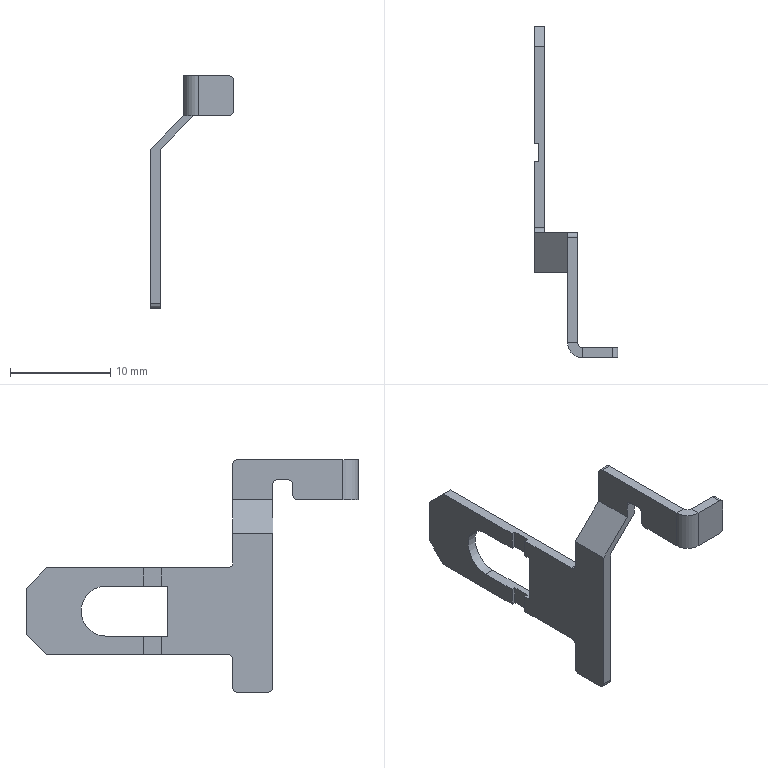Part | SolidWorks | features ICE 5, Chamfer 1, Fillet 1, FlatPattern 1, SMBaseFlange 1, SheetMetal 1 | 1 solid | 49 faces | box 8.33 x 33.1 x 23.2 mm | volume 267.226 mm3 | plane 36 | cylinder 13 | commonest cylinder face diameters 1 x11 3 x1 5 x1
STEP:
#1=CARTESIAN_POINT('',(-8.33,21.4,-8.6));
#2=VERTEX_POINT('',#1);
#3=CARTESIAN_POINT('',(-8.33,21.4,-6.8));
#4=VERTEX_POINT('',#3);
#5=CARTESIAN_POINT('',(-8.33,21.4,-19.2));
#6=DIRECTION('',(0.,0.,1.));
#7=VECTOR('',#6,1000.);
#8=LINE('',#5,#7);
#9=EDGE_CURVE('',#2,#4,#8,.T.);
#10=ORIENTED_EDGE('',*,*,#9,.F.);
#11=CARTESIAN_POINT('',(-7.93,21.4,-8.6));
#12=VERTEX_POINT('',#11);
#13=CARTESIAN_POINT('',(-8.33,21.4,-8.6));
#14=DIRECTION('',(1.,0.,0.));
#15=VECTOR('',#14,1000.);
#16=LINE('',#13,#15);
#17=EDGE_CURVE('',#2,#12,#16,.T.);
#18=ORIENTED_EDGE('',*,*,#17,.T.);
#19=CARTESIAN_POINT('',(-7.93,21.4,-6.8));
#20=VERTEX_POINT('',#19);
#21=CARTESIAN_POINT('',(-7.93,21.4,-19.2));
#22=DIRECTION('',(0.,0.,1.));
#23=VECTOR('',#22,1000.);
#24=LINE('',#21,#23);
#25=EDGE_CURVE('',#12,#20,#24,.T.);
#26=ORIENTED_EDGE('',*,*,#25,.T.);
#27=CARTESIAN_POINT('',(-8.33,21.4,-6.8));
#28=DIRECTION('',(-1.,0.,0.));
#29=VECTOR('',#28,1000.);
#30=LINE('',#27,#29);
#31=EDGE_CURVE('',#20,#4,#30,.T.);
#32=ORIENTED_EDGE('',*,*,#31,.T.);
#33=EDGE_LOOP('',(#10,#18,#26,#32));
#34=FACE_OUTER_BOUND('',#33,.T.);
#35=CARTESIAN_POINT('',(-8.33,21.4,-19.2));
#36=DIRECTION('',(0.,1.,0.));
#37=DIRECTION('',(-1.,0.,0.));
#38=AXIS2_PLACEMENT_3D('',#35,#36,#37);
#39=PLANE('',#38);
#40=ADVANCED_FACE('',(#34),#39,.F.);
#41=ORIENTED_EDGE('',*,*,#25,.F.);
#42=CARTESIAN_POINT('',(-7.93,19.6,-8.6));
#43=VERTEX_POINT('',#42);
#44=CARTESIAN_POINT('',(-7.93,21.4,-8.6));
#45=DIRECTION('',(0.,-1.,0.));
#46=VECTOR('',#45,1000.);
#47=LINE('',#44,#46);
#48=EDGE_CURVE('',#12,#43,#47,.T.);
#49=ORIENTED_EDGE('',*,*,#48,.T.);
#50=CARTESIAN_POINT('',(-7.93,19.6,-6.8));
#51=VERTEX_POINT('',#50);
#52=CARTESIAN_POINT('',(-7.93,19.6,-19.2));
#53=DIRECTION('',(0.,0.,1.));
#54=VECTOR('',#53,1000.);
#55=LINE('',#52,#54);
#56=EDGE_CURVE('',#43,#51,#55,.T.);
#57=ORIENTED_EDGE('',*,*,#56,.T.);
#58=CARTESIAN_POINT('',(-7.93,21.4,-6.8));
#59=DIRECTION('',(0.,1.,0.));
#60=VECTOR('',#59,1000.);
#61=LINE('',#58,#60);
#62=EDGE_CURVE('',#51,#20,#61,.T.);
#63=ORIENTED_EDGE('',*,*,#62,.T.);
#64=EDGE_LOOP('',(#41,#49,#57,#63));
#65=FACE_OUTER_BOUND('',#64,.T.);
#66=CARTESIAN_POINT('',(-7.93,21.4,-19.2));
#67=DIRECTION('',(1.,0.,0.));
#68=DIRECTION('',(0.,0.,-1.));
#69=AXIS2_PLACEMENT_3D('',#66,#67,#68);
#70=PLANE('',#69);
#71=ADVANCED_FACE('',(#65),#70,.F.);
#72=ORIENTED_EDGE('',*,*,#56,.F.);
#73=CARTESIAN_POINT('',(-8.33,19.6,-8.6));
#74=VERTEX_POINT('',#73);
#75=CARTESIAN_POINT('',(-8.33,19.6,-8.6));
#76=DIRECTION('',(-1.,0.,0.));
#77=VECTOR('',#76,1000.);
#78=LINE('',#75,#77);
#79=EDGE_CURVE('',#43,#74,#78,.T.);
#80=ORIENTED_EDGE('',*,*,#79,.T.);
#81=CARTESIAN_POINT('',(-8.33,19.6,-6.8));
#82=VERTEX_POINT('',#81);
#83=CARTESIAN_POINT('',(-8.33,19.6,-19.2));
#84=DIRECTION('',(0.,0.,1.));
#85=VECTOR('',#84,1000.);
#86=LINE('',#83,#85);
#87=EDGE_CURVE('',#74,#82,#86,.T.);
#88=ORIENTED_EDGE('',*,*,#87,.T.);
#89=CARTESIAN_POINT('',(-8.33,19.6,-6.8));
#90=DIRECTION('',(1.,0.,0.));
#91=VECTOR('',#90,1000.);
#92=LINE('',#89,#91);
#93=EDGE_CURVE('',#82,#51,#92,.T.);
#94=ORIENTED_EDGE('',*,*,#93,.T.);
#95=EDGE_LOOP('',(#72,#80,#88,#94));
#96=FACE_OUTER_BOUND('',#95,.T.);
#97=CARTESIAN_POINT('',(-8.33,19.6,-19.2));
#98=DIRECTION('',(0.,-1.,0.));
#99=DIRECTION('',(0.,0.,-1.));
#100=AXIS2_PLACEMENT_3D('',#97,#98,#99);
#101=PLANE('',#100);
#102=ADVANCED_FACE('',(#96),#101,.F.);
#103=CARTESIAN_POINT('',(-8.33,31.1,-6.8));
#104=VERTEX_POINT('',#103);
#105=CARTESIAN_POINT('',(-8.33,12.5,-6.8));
#106=DIRECTION('',(0.,1.,0.));
#107=VECTOR('',#106,1000.);
#108=LINE('',#105,#107);
#109=EDGE_CURVE('',#4,#104,#108,.T.);
#110=ORIENTED_EDGE('',*,*,#109,.T.);
#111=CARTESIAN_POINT('',(-8.33,33.1,-8.8));
#112=VERTEX_POINT('',#111);
#113=CARTESIAN_POINT('',(-8.33,26.,-1.7));
#114=DIRECTION('',(0.,0.7071,-0.7071));
#115=VECTOR('',#114,1000.);
#116=LINE('',#113,#115);
#117=EDGE_CURVE('',#104,#112,#116,.T.);
#118=ORIENTED_EDGE('',*,*,#117,.T.);
#119=CARTESIAN_POINT('',(-8.33,33.1,-13.4));
#120=VERTEX_POINT('',#119);
#121=CARTESIAN_POINT('',(-8.33,33.1,-15.4));
#122=DIRECTION('',(0.,0.,-1.));
#123=VECTOR('',#122,1000.);
#124=LINE('',#121,#123);
#125=EDGE_CURVE('',#112,#120,#124,.T.);
#126=ORIENTED_EDGE('',*,*,#125,.T.);
#127=CARTESIAN_POINT('',(-8.33,31.1,-15.4));
#128=VERTEX_POINT('',#127);
#129=CARTESIAN_POINT('',(-8.33,17.9,-28.6));
#130=DIRECTION('',(0.,-0.7071,-0.7071));
#131=VECTOR('',#130,1000.);
#132=LINE('',#129,#131);
#133=EDGE_CURVE('',#120,#128,#132,.T.);
#134=ORIENTED_EDGE('',*,*,#133,.T.);
#135=CARTESIAN_POINT('',(-8.33,21.4,-15.4));
#136=VERTEX_POINT('',#135);
#137=CARTESIAN_POINT('',(-8.33,12.5,-15.4));
#138=DIRECTION('',(0.,-1.,0.));
#139=VECTOR('',#138,1000.);
#140=LINE('',#137,#139);
#141=EDGE_CURVE('',#128,#136,#140,.T.);
#142=ORIENTED_EDGE('',*,*,#141,.T.);
#143=CARTESIAN_POINT('',(-8.33,21.4,-13.6));
#144=VERTEX_POINT('',#143);
#145=CARTESIAN_POINT('',(-8.33,21.4,-19.2));
#146=DIRECTION('',(0.,0.,1.));
#147=VECTOR('',#146,1000.);
#148=LINE('',#145,#147);
#149=EDGE_CURVE('',#136,#144,#148,.T.);
#150=ORIENTED_EDGE('',*,*,#149,.T.);
#151=CARTESIAN_POINT('',(-8.33,25.1,-13.6));
#152=VERTEX_POINT('',#151);
#153=CARTESIAN_POINT('',(-8.33,25.1,-13.6));
#154=DIRECTION('',(0.,-1.,0.));
#155=VECTOR('',#154,1000.);
#156=LINE('',#153,#155);
#157=EDGE_CURVE('',#152,#144,#156,.T.);
#158=ORIENTED_EDGE('',*,*,#157,.F.);
#159=CARTESIAN_POINT('',(-8.33,25.1,-8.6));
#160=VERTEX_POINT('',#159);
#161=CARTESIAN_POINT('',(-8.33,25.1,-11.1));
#162=DIRECTION('',(-1.,0.,0.));
#163=DIRECTION('',(0.,0.,1.));
#164=AXIS2_PLACEMENT_3D('',#161,#162,#163);
#165=CIRCLE('',#164,2.5);
#166=EDGE_CURVE('',#160,#152,#165,.T.);
#167=ORIENTED_EDGE('',*,*,#166,.F.);
#168=CARTESIAN_POINT('',(-8.33,25.1,-8.6));
#169=DIRECTION('',(0.,1.,0.));
#170=VECTOR('',#169,1000.);
#171=LINE('',#168,#170);
#172=EDGE_CURVE('',#2,#160,#171,.T.);
#173=ORIENTED_EDGE('',*,*,#172,.F.);
#174=ORIENTED_EDGE('',*,*,#9,.T.);
#175=EDGE_LOOP('',(#110,#118,#126,#134,#142,#150,#158,#167,#173,#174));
#176=FACE_OUTER_BOUND('',#175,.T.);
#177=CARTESIAN_POINT('',(-8.33,8.5,-19.2));
#178=DIRECTION('',(-1.,0.,0.));
#179=DIRECTION('',(0.,0.,1.));
#180=AXIS2_PLACEMENT_3D('',#177,#178,#179);
#181=PLANE('',#180);
#182=ADVANCED_FACE('',(#176),#181,.T.);
#183=CARTESIAN_POINT('',(-7.33,12.5,-3.33));
#184=VERTEX_POINT('',#183);
#185=CARTESIAN_POINT('',(-7.33,12.5,-6.3));
#186=VERTEX_POINT('',#185);
#187=CARTESIAN_POINT('',(-7.33,12.5,-3.33));
#188=DIRECTION('',(0.,0.,-1.));
#189=VECTOR('',#188,1000.);
#190=LINE('',#187,#189);
#191=EDGE_CURVE('',#184,#186,#190,.T.);
#192=ORIENTED_EDGE('',*,*,#191,.T.);
#193=CARTESIAN_POINT('',(-8.33,12.5,-6.3));
#194=VERTEX_POINT('',#193);
#195=CARTESIAN_POINT('',(-8.33,12.5,-6.3));
#196=DIRECTION('',(-1.,0.,0.));
#197=VECTOR('',#196,1000.);
#198=LINE('',#195,#197);
#199=EDGE_CURVE('',#186,#194,#198,.T.);
#200=ORIENTED_EDGE('',*,*,#199,.T.);
#201=CARTESIAN_POINT('',(-8.33,12.5,-3.33));
#202=VERTEX_POINT('',#201);
#203=CARTESIAN_POINT('',(-8.33,12.5,-19.2));
#204=DIRECTION('',(0.,0.,1.));
#205=VECTOR('',#204,1000.);
#206=LINE('',#203,#205);
#207=EDGE_CURVE('',#194,#202,#206,.T.);
#208=ORIENTED_EDGE('',*,*,#207,.T.);
#209=CARTESIAN_POINT('',(-5.,12.5,0.));
#210=VERTEX_POINT('',#209);
#211=CARTESIAN_POINT('',(-8.33,12.5,-3.33));
#212=DIRECTION('',(0.7071,0.,0.7071));
#213=VECTOR('',#212,1000.);
#214=LINE('',#211,#213);
#215=EDGE_CURVE('',#202,#210,#214,.T.);
#216=ORIENTED_EDGE('',*,*,#215,.T.);
#217=CARTESIAN_POINT('',(-5.,12.5,3.5));
#218=VERTEX_POINT('',#217);
#219=CARTESIAN_POINT('',(-5.,12.5,4.));
#220=DIRECTION('',(0.,0.,-1.));
#221=VECTOR('',#220,1000.);
#222=LINE('',#219,#221);
#223=EDGE_CURVE('',#218,#210,#222,.T.);
#224=ORIENTED_EDGE('',*,*,#223,.F.);
#225=CARTESIAN_POINT('',(-4.,12.5,3.5));
#226=VERTEX_POINT('',#225);
#227=CARTESIAN_POINT('',(-5.,12.5,3.5));
#228=DIRECTION('',(1.,0.,0.));
#229=VECTOR('',#228,1000.);
#230=LINE('',#227,#229);
#231=EDGE_CURVE('',#218,#226,#230,.T.);
#232=ORIENTED_EDGE('',*,*,#231,.T.);
#233=CARTESIAN_POINT('',(-4.,12.5,0.));
#234=VERTEX_POINT('',#233);
#235=CARTESIAN_POINT('',(-4.,12.5,4.));
#236=DIRECTION('',(0.,0.,-1.));
#237=VECTOR('',#236,1000.);
#238=LINE('',#235,#237);
#239=EDGE_CURVE('',#226,#234,#238,.T.);
#240=ORIENTED_EDGE('',*,*,#239,.T.);
#241=CARTESIAN_POINT('',(-4.,12.5,0.));
#242=DIRECTION('',(-0.7071,0.,-0.7071));
#243=VECTOR('',#242,1000.);
#244=LINE('',#241,#243);
#245=EDGE_CURVE('',#234,#184,#244,.T.);
#246=ORIENTED_EDGE('',*,*,#245,.T.);
#247=EDGE_LOOP('',(#192,#200,#208,#216,#224,#232,#240,#246));
#248=FACE_OUTER_BOUND('',#247,.T.);
#249=CARTESIAN_POINT('',(-5.,12.5,4.));
#250=DIRECTION('',(0.,1.,0.));
#251=DIRECTION('',(0.,0.,1.));
#252=AXIS2_PLACEMENT_3D('',#249,#250,#251);
#253=PLANE('',#252);
#254=ADVANCED_FACE('',(#248),#253,.T.);
#255=CARTESIAN_POINT('',(-5.,1.5,0.));
#256=VERTEX_POINT('',#255);
#257=CARTESIAN_POINT('',(-5.,6.,0.));
#258=VERTEX_POINT('',#257);
#259=CARTESIAN_POINT('',(-5.,0.,0.));
#260=DIRECTION('',(0.,1.,0.));
#261=VECTOR('',#260,1000.);
#262=LINE('',#259,#261);
#263=EDGE_CURVE('',#256,#258,#262,.T.);
#264=ORIENTED_EDGE('',*,*,#263,.T.);
#265=CARTESIAN_POINT('',(-4.,6.,0.));
#266=VERTEX_POINT('',#265);
#267=CARTESIAN_POINT('',(-3.5,6.,0.));
#268=DIRECTION('',(1.,0.,0.));
#269=VECTOR('',#268,1000.);
#270=LINE('',#267,#269);
#271=EDGE_CURVE('',#258,#266,#270,.T.);
#272=ORIENTED_EDGE('',*,*,#271,.T.);
#273=CARTESIAN_POINT('',(-4.,1.5,0.));
#274=VERTEX_POINT('',#273);
#275=CARTESIAN_POINT('',(-4.,0.,0.));
#276=DIRECTION('',(0.,1.,0.));
#277=VECTOR('',#276,1000.);
#278=LINE('',#275,#277);
#279=EDGE_CURVE('',#274,#266,#278,.T.);
#280=ORIENTED_EDGE('',*,*,#279,.F.);
#281=CARTESIAN_POINT('',(-4.,1.5,0.));
#282=DIRECTION('',(-1.,0.,0.));
#283=VECTOR('',#282,1000.);
#284=LINE('',#281,#283);
#285=EDGE_CURVE('',#274,#256,#284,.T.);
#286=ORIENTED_EDGE('',*,*,#285,.T.);
#287=EDGE_LOOP('',(#264,#272,#280,#286));
#288=FACE_OUTER_BOUND('',#287,.T.);
#289=CARTESIAN_POINT('',(-3.5,1.5,0.));
#290=DIRECTION('',(0.,0.,1.));
#291=DIRECTION('',(1.,0.,0.));
#292=AXIS2_PLACEMENT_3D('',#289,#290,#291);
#293=PLANE('',#292);
#294=ADVANCED_FACE('',(#288),#293,.F.);
#295=CARTESIAN_POINT('',(-5.,1.5,4.));
#296=VERTEX_POINT('',#295);
#297=CARTESIAN_POINT('',(-4.,1.5,4.));
#298=VERTEX_POINT('',#297);
#299=CARTESIAN_POINT('',(-5.,1.5,4.));
#300=DIRECTION('',(1.,0.,0.));
#301=VECTOR('',#300,1000.);
#302=LINE('',#299,#301);
#303=EDGE_CURVE('',#296,#298,#302,.T.);
#304=ORIENTED_EDGE('',*,*,#303,.F.);
#305=CARTESIAN_POINT('',(-3.5,0.,4.));
#306=VERTEX_POINT('',#305);
#307=CARTESIAN_POINT('',(-3.5,1.5,4.));
#308=DIRECTION('',(0.,0.,-1.));
#309=DIRECTION('',(1.,0.,0.));
#310=AXIS2_PLACEMENT_3D('',#307,#308,#309);
#311=CIRCLE('',#310,1.5);
#312=EDGE_CURVE('',#306,#296,#311,.T.);
#313=ORIENTED_EDGE('',*,*,#312,.F.);
#314=CARTESIAN_POINT('',(-3.5,1.,4.));
#315=VERTEX_POINT('',#314);
#316=CARTESIAN_POINT('',(-3.5,1.,4.));
#317=DIRECTION('',(0.,-1.,0.));
#318=VECTOR('',#317,1000.);
#319=LINE('',#316,#318);
#320=EDGE_CURVE('',#315,#306,#319,.T.);
#321=ORIENTED_EDGE('',*,*,#320,.F.);
#322=CARTESIAN_POINT('',(-3.5,1.5,4.));
#323=DIRECTION('',(0.,0.,-1.));
#324=DIRECTION('',(1.,0.,0.));
#325=AXIS2_PLACEMENT_3D('',#322,#323,#324);
#326=CIRCLE('',#325,0.5);
#327=EDGE_CURVE('',#315,#298,#326,.T.);
#328=ORIENTED_EDGE('',*,*,#327,.T.);
#329=EDGE_LOOP('',(#304,#313,#321,#328));
#330=FACE_OUTER_BOUND('',#329,.T.);
#331=CARTESIAN_POINT('',(-5.,1.5,4.));
#332=DIRECTION('',(0.,0.,1.));
#333=DIRECTION('',(1.,0.,0.));
#334=AXIS2_PLACEMENT_3D('',#331,#332,#333);
#335=PLANE('',#334);
#336=ADVANCED_FACE('',(#330),#335,.T.);
#337=CARTESIAN_POINT('',(-4.,12.,4.));
#338=VERTEX_POINT('',#337);
#339=CARTESIAN_POINT('',(-4.,0.,4.));
#340=DIRECTION('',(0.,1.,0.));
#341=VECTOR('',#340,1000.);
#342=LINE('',#339,#341);
#343=EDGE_CURVE('',#298,#338,#342,.T.);
#344=ORIENTED_EDGE('',*,*,#343,.T.);
#345=CARTESIAN_POINT('',(-5.,12.,4.));
#346=VERTEX_POINT('',#345);
#347=CARTESIAN_POINT('',(-3.5,12.,4.));
#348=DIRECTION('',(-1.,0.,0.));
#349=VECTOR('',#348,1000.);
#350=LINE('',#347,#349);
#351=EDGE_CURVE('',#338,#346,#350,.T.);
#352=ORIENTED_EDGE('',*,*,#351,.T.);
#353=CARTESIAN_POINT('',(-5.,0.,4.));
#354=DIRECTION('',(0.,1.,0.));
#355=VECTOR('',#354,1000.);
#356=LINE('',#353,#355);
#357=EDGE_CURVE('',#296,#346,#356,.T.);
#358=ORIENTED_EDGE('',*,*,#357,.F.);
#359=ORIENTED_EDGE('',*,*,#303,.T.);
#360=EDGE_LOOP('',(#344,#352,#358,#359));
#361=FACE_OUTER_BOUND('',#360,.T.);
#362=CARTESIAN_POINT('',(-3.5,1.,4.));
#363=DIRECTION('',(0.,0.,1.));
#364=DIRECTION('',(1.,0.,0.));
#365=AXIS2_PLACEMENT_3D('',#362,#363,#364);
#366=PLANE('',#365);
#367=ADVANCED_FACE('',(#361),#366,.T.);
#368=CARTESIAN_POINT('',(-3.5,0.,0.));
#369=VERTEX_POINT('',#368);
#370=CARTESIAN_POINT('',(-3.5,1.,0.));
#371=VERTEX_POINT('',#370);
#372=CARTESIAN_POINT('',(-3.5,0.,0.));
#373=DIRECTION('',(0.,1.,0.));
#374=VECTOR('',#373,1000.);
#375=LINE('',#372,#374);
#376=EDGE_CURVE('',#369,#371,#375,.T.);
#377=ORIENTED_EDGE('',*,*,#376,.F.);
#378=CARTESIAN_POINT('',(-3.5,1.5,0.));
#379=DIRECTION('',(0.,0.,-1.));
#380=DIRECTION('',(1.,0.,0.));
#381=AXIS2_PLACEMENT_3D('',#378,#379,#380);
#382=CIRCLE('',#381,1.5);
#383=EDGE_CURVE('',#369,#256,#382,.T.);
#384=ORIENTED_EDGE('',*,*,#383,.T.);
#385=ORIENTED_EDGE('',*,*,#285,.F.);
#386=CARTESIAN_POINT('',(-3.5,1.5,0.));
#387=DIRECTION('',(0.,0.,-1.));
#388=DIRECTION('',(1.,0.,0.));
#389=AXIS2_PLACEMENT_3D('',#386,#387,#388);
#390=CIRCLE('',#389,0.5);
#391=EDGE_CURVE('',#371,#274,#390,.T.);
#392=ORIENTED_EDGE('',*,*,#391,.F.);
#393=EDGE_LOOP('',(#377,#384,#385,#392));
#394=FACE_OUTER_BOUND('',#393,.T.);
#395=CARTESIAN_POINT('',(-3.5,0.,0.));
#396=DIRECTION('',(0.,0.,-1.));
#397=DIRECTION('',(-1.,0.,0.));
#398=AXIS2_PLACEMENT_3D('',#395,#396,#397);
#399=PLANE('',#398);
#400=ADVANCED_FACE('',(#394),#399,.T.);
#401=CARTESIAN_POINT('',(-0.5,1.,0.));
#402=VERTEX_POINT('',#401);
#403=CARTESIAN_POINT('',(0.,1.,0.));
#404=DIRECTION('',(-1.,0.,0.));
#405=VECTOR('',#404,1000.);
#406=LINE('',#403,#405);
#407=EDGE_CURVE('',#402,#371,#406,.T.);
#408=ORIENTED_EDGE('',*,*,#407,.F.);
#409=CARTESIAN_POINT('',(-0.5,0.,0.));
#410=VERTEX_POINT('',#409);
#411=CARTESIAN_POINT('',(-0.5,1.5,0.));
#412=DIRECTION('',(0.,-1.,0.));
#413=VECTOR('',#412,1000.);
#414=LINE('',#411,#413);
#415=EDGE_CURVE('',#402,#410,#414,.T.);
#416=ORIENTED_EDGE('',*,*,#415,.T.);
#417=CARTESIAN_POINT('',(0.,0.,0.));
#418=DIRECTION('',(-1.,0.,0.));
#419=VECTOR('',#418,1000.);
#420=LINE('',#417,#419);
#421=EDGE_CURVE('',#410,#369,#420,.T.);
#422=ORIENTED_EDGE('',*,*,#421,.T.);
#423=ORIENTED_EDGE('',*,*,#376,.T.);
#424=EDGE_LOOP('',(#408,#416,#422,#423));
#425=FACE_OUTER_BOUND('',#424,.T.);
#426=CARTESIAN_POINT('',(-4.,1.5,0.));
#427=DIRECTION('',(0.,0.,-1.));
#428=DIRECTION('',(-1.,0.,0.));
#429=AXIS2_PLACEMENT_3D('',#426,#427,#428);
#430=PLANE('',#429);
#431=ADVANCED_FACE('',(#425),#430,.T.);
#432=ORIENTED_EDGE('',*,*,#279,.T.);
#433=CARTESIAN_POINT('',(-4.,6.5,0.5));
#434=VERTEX_POINT('',#433);
#435=CARTESIAN_POINT('',(-4.,6.,0.5));
#436=DIRECTION('',(1.,0.,0.));
#437=DIRECTION('',(0.,0.,1.));
#438=AXIS2_PLACEMENT_3D('',#435,#436,#437);
#439=CIRCLE('',#438,0.5);
#440=EDGE_CURVE('',#266,#434,#439,.T.);
#441=ORIENTED_EDGE('',*,*,#440,.T.);
#442=CARTESIAN_POINT('',(-4.,6.5,1.5));
#443=VERTEX_POINT('',#442);
#444=CARTESIAN_POINT('',(-4.,6.5,4.));
#445=DIRECTION('',(0.,0.,1.));
#446=VECTOR('',#445,1000.);
#447=LINE('',#444,#446);
#448=EDGE_CURVE('',#434,#443,#447,.T.);
#449=ORIENTED_EDGE('',*,*,#448,.T.);
#450=CARTESIAN_POINT('',(-4.,7.,2.));
#451=VERTEX_POINT('',#450);
#452=CARTESIAN_POINT('',(-4.,7.,1.5));
#453=DIRECTION('',(-1.,0.,0.));
#454=DIRECTION('',(0.,0.,1.));
#455=AXIS2_PLACEMENT_3D('',#452,#453,#454);
#456=CIRCLE('',#455,0.5);
#457=EDGE_CURVE('',#443,#451,#456,.T.);
#458=ORIENTED_EDGE('',*,*,#457,.T.);
#459=CARTESIAN_POINT('',(-4.,8.,2.));
#460=VERTEX_POINT('',#459);
#461=CARTESIAN_POINT('',(-4.,0.,2.));
#462=DIRECTION('',(0.,1.,0.));
#463=VECTOR('',#462,1000.);
#464=LINE('',#461,#463);
#465=EDGE_CURVE('',#451,#460,#464,.T.);
#466=ORIENTED_EDGE('',*,*,#465,.T.);
#467=CARTESIAN_POINT('',(-4.,8.5,1.5));
#468=VERTEX_POINT('',#467);
#469=CARTESIAN_POINT('',(-4.,8.,1.5));
#470=DIRECTION('',(-1.,0.,0.));
#471=DIRECTION('',(0.,0.,1.));
#472=AXIS2_PLACEMENT_3D('',#469,#470,#471);
#473=CIRCLE('',#472,0.5);
#474=EDGE_CURVE('',#460,#468,#473,.T.);
#475=ORIENTED_EDGE('',*,*,#474,.T.);
#476=CARTESIAN_POINT('',(-4.,8.5,0.));
#477=VERTEX_POINT('',#476);
#478=CARTESIAN_POINT('',(-4.,8.5,4.));
#479=DIRECTION('',(0.,0.,-1.));
#480=VECTOR('',#479,1000.);
#481=LINE('',#478,#480);
#482=EDGE_CURVE('',#468,#477,#481,.T.);
#483=ORIENTED_EDGE('',*,*,#482,.T.);
#484=CARTESIAN_POINT('',(-4.,8.5,0.));
#485=DIRECTION('',(0.,1.,0.));
#486=VECTOR('',#485,1000.);
#487=LINE('',#484,#486);
#488=EDGE_CURVE('',#477,#234,#487,.T.);
#489=ORIENTED_EDGE('',*,*,#488,.T.);
#490=ORIENTED_EDGE('',*,*,#239,.F.);
#491=CARTESIAN_POINT('',(-4.,12.,3.5));
#492=DIRECTION('',(1.,0.,0.));
#493=DIRECTION('',(0.,0.,1.));
#494=AXIS2_PLACEMENT_3D('',#491,#492,#493);
#495=CIRCLE('',#494,0.5);
#496=EDGE_CURVE('',#226,#338,#495,.T.);
#497=ORIENTED_EDGE('',*,*,#496,.T.);
#498=ORIENTED_EDGE('',*,*,#343,.F.);
#499=CARTESIAN_POINT('',(-4.,1.5,4.));
#500=DIRECTION('',(0.,0.,-1.));
#501=VECTOR('',#500,1000.);
#502=LINE('',#499,#501);
#503=EDGE_CURVE('',#298,#274,#502,.T.);
#504=ORIENTED_EDGE('',*,*,#503,.T.);
#505=EDGE_LOOP('',(#432,#441,#449,#458,#466,#475,#483,#489,#490,#497,#498,#504));
#506=FACE_OUTER_BOUND('',#505,.T.);
#507=CARTESIAN_POINT('',(-4.,0.,4.));
#508=DIRECTION('',(-1.,0.,0.));
#509=DIRECTION('',(0.,0.,1.));
#510=AXIS2_PLACEMENT_3D('',#507,#508,#509);
#511=PLANE('',#510);
#512=ADVANCED_FACE('',(#506),#511,.F.);
#513=CARTESIAN_POINT('',(-8.33,12.5,-18.7));
#514=VERTEX_POINT('',#513);
#515=CARTESIAN_POINT('',(-8.33,12.5,-15.9));
#516=VERTEX_POINT('',#515);
#517=CARTESIAN_POINT('',(-8.33,12.5,-19.2));
#518=DIRECTION('',(0.,0.,1.));
#519=VECTOR('',#518,1000.);
#520=LINE('',#517,#519);
#521=EDGE_CURVE('',#514,#516,#520,.T.);
#522=ORIENTED_EDGE('',*,*,#521,.T.);
#523=CARTESIAN_POINT('',(-7.33,12.5,-15.9));
#524=VERTEX_POINT('',#523);
#525=CARTESIAN_POINT('',(-7.33,12.5,-15.9));
#526=DIRECTION('',(1.,0.,0.));
#527=VECTOR('',#526,1000.);
#528=LINE('',#525,#527);
#529=EDGE_CURVE('',#516,#524,#528,.T.);
#530=ORIENTED_EDGE('',*,*,#529,.T.);
#531=CARTESIAN_POINT('',(-7.33,12.5,-18.7));
#532=VERTEX_POINT('',#531);
#533=CARTESIAN_POINT('',(-7.33,12.5,-3.33));
#534=DIRECTION('',(0.,0.,-1.));
#535=VECTOR('',#534,1000.);
#536=LINE('',#533,#535);
#537=EDGE_CURVE('',#524,#532,#536,.T.);
#538=ORIENTED_EDGE('',*,*,#537,.T.);
#539=CARTESIAN_POINT('',(-5.,12.5,-18.7));
#540=DIRECTION('',(-1.,0.,0.));
#541=VECTOR('',#540,1000.);
#542=LINE('',#539,#541);
#543=EDGE_CURVE('',#532,#514,#542,.T.);
#544=ORIENTED_EDGE('',*,*,#543,.T.);
#545=EDGE_LOOP('',(#522,#530,#538,#544));
#546=FACE_OUTER_BOUND('',#545,.T.);
#547=CARTESIAN_POINT('',(-5.,12.5,4.));
#548=DIRECTION('',(0.,1.,0.));
#549=DIRECTION('',(0.,0.,1.));
#550=AXIS2_PLACEMENT_3D('',#547,#548,#549);
#551=PLANE('',#550);
#552=ADVANCED_FACE('',(#546),#551,.T.);
#553=CARTESIAN_POINT('',(-5.,6.5,0.5));
#554=VERTEX_POINT('',#553);
#555=CARTESIAN_POINT('',(-5.,6.5,1.5));
#556=VERTEX_POINT('',#555);
#557=CARTESIAN_POINT('',(-5.,6.5,0.));
#558=DIRECTION('',(0.,0.,1.));
#559=VECTOR('',#558,1000.);
#560=LINE('',#557,#559);
#561=EDGE_CURVE('',#554,#556,#560,.T.);
#562=ORIENTED_EDGE('',*,*,#561,.F.);
#563=CARTESIAN_POINT('',(-5.,6.,0.5));
#564=DIRECTION('',(-1.,0.,0.));
#565=DIRECTION('',(0.,0.,1.));
#566=AXIS2_PLACEMENT_3D('',#563,#564,#565);
#567=CIRCLE('',#566,0.5);
#568=EDGE_CURVE('',#554,#258,#567,.T.);
#569=ORIENTED_EDGE('',*,*,#568,.T.);
#570=ORIENTED_EDGE('',*,*,#263,.F.);
#571=CARTESIAN_POINT('',(-5.,1.5,4.));
#572=DIRECTION('',(0.,0.,-1.));
#573=VECTOR('',#572,1000.);
#574=LINE('',#571,#573);
#575=EDGE_CURVE('',#296,#256,#574,.T.);
#576=ORIENTED_EDGE('',*,*,#575,.F.);
#577=ORIENTED_EDGE('',*,*,#357,.T.);
#578=CARTESIAN_POINT('',(-5.,12.,3.5));
#579=DIRECTION('',(-1.,0.,0.));
#580=DIRECTION('',(0.,0.,1.));
#581=AXIS2_PLACEMENT_3D('',#578,#579,#580);
#582=CIRCLE('',#581,0.5);
#583=EDGE_CURVE('',#346,#218,#582,.T.);
#584=ORIENTED_EDGE('',*,*,#583,.T.);
#585=ORIENTED_EDGE('',*,*,#223,.T.);
#586=CARTESIAN_POINT('',(-5.,8.5,0.));
#587=VERTEX_POINT('',#586);
#588=CARTESIAN_POINT('',(-5.,8.5,0.));
#589=DIRECTION('',(0.,1.,0.));
#590=VECTOR('',#589,1000.);
#591=LINE('',#588,#590);
#592=EDGE_CURVE('',#587,#210,#591,.T.);
#593=ORIENTED_EDGE('',*,*,#592,.F.);
#594=CARTESIAN_POINT('',(-5.,8.5,1.5));
#595=VERTEX_POINT('',#594);
#596=CARTESIAN_POINT('',(-5.,8.5,0.));
#597=DIRECTION('',(0.,0.,-1.));
#598=VECTOR('',#597,1000.);
#599=LINE('',#596,#598);
#600=EDGE_CURVE('',#595,#587,#599,.T.);
#601=ORIENTED_EDGE('',*,*,#600,.F.);
#602=CARTESIAN_POINT('',(-5.,8.,2.));
#603=VERTEX_POINT('',#602);
#604=CARTESIAN_POINT('',(-5.,8.,1.5));
#605=DIRECTION('',(1.,0.,0.));
#606=DIRECTION('',(0.,0.,1.));
#607=AXIS2_PLACEMENT_3D('',#604,#605,#606);
#608=CIRCLE('',#607,0.5);
#609=EDGE_CURVE('',#595,#603,#608,.T.);
#610=ORIENTED_EDGE('',*,*,#609,.T.);
#611=CARTESIAN_POINT('',(-5.,7.,2.));
#612=VERTEX_POINT('',#611);
#613=CARTESIAN_POINT('',(-5.,8.5,2.));
#614=DIRECTION('',(0.,1.,0.));
#615=VECTOR('',#614,1000.);
#616=LINE('',#613,#615);
#617=EDGE_CURVE('',#612,#603,#616,.T.);
#618=ORIENTED_EDGE('',*,*,#617,.F.);
#619=CARTESIAN_POINT('',(-5.,7.,1.5));
#620=DIRECTION('',(1.,0.,0.));
#621=DIRECTION('',(0.,0.,1.));
#622=AXIS2_PLACEMENT_3D('',#619,#620,#621);
#623=CIRCLE('',#622,0.5);
#624=EDGE_CURVE('',#612,#556,#623,.T.);
#625=ORIENTED_EDGE('',*,*,#624,.T.);
#626=EDGE_LOOP('',(#562,#569,#570,#576,#577,#584,#585,#593,#601,#610,#618,#625));
#627=FACE_OUTER_BOUND('',#626,.T.);
#628=CARTESIAN_POINT('',(-5.,0.,4.));
#629=DIRECTION('',(-1.,0.,0.));
#630=DIRECTION('',(0.,0.,1.));
#631=AXIS2_PLACEMENT_3D('',#628,#629,#630);
#632=PLANE('',#631);
#633=ADVANCED_FACE('',(#627),#632,.T.);
#634=ORIENTED_EDGE('',*,*,#383,.F.);
#635=CARTESIAN_POINT('',(-3.5,0.,4.));
#636=DIRECTION('',(0.,0.,-1.));
#637=VECTOR('',#636,1000.);
#638=LINE('',#635,#637);
#639=EDGE_CURVE('',#306,#369,#638,.T.);
#640=ORIENTED_EDGE('',*,*,#639,.F.);
#641=ORIENTED_EDGE('',*,*,#312,.T.);
#642=ORIENTED_EDGE('',*,*,#575,.T.);
#643=EDGE_LOOP('',(#634,#640,#641,#642));
#644=FACE_OUTER_BOUND('',#643,.T.);
#645=CARTESIAN_POINT('',(-3.5,1.5,4.));
#646=DIRECTION('',(0.,0.,-1.));
#647=DIRECTION('',(-1.,0.,0.));
#648=AXIS2_PLACEMENT_3D('',#645,#646,#647);
#649=CYLINDRICAL_SURFACE('',#648,1.5);
#650=ADVANCED_FACE('',(#644),#649,.T.);
#651=CARTESIAN_POINT('',(0.,0.,3.5));
#652=VERTEX_POINT('',#651);
#653=CARTESIAN_POINT('',(0.,0.,0.5));
#654=VERTEX_POINT('',#653);
#655=CARTESIAN_POINT('',(0.,0.,4.));
#656=DIRECTION('',(0.,0.,-1.));
#657=VECTOR('',#656,1000.);
#658=LINE('',#655,#657);
#659=EDGE_CURVE('',#652,#654,#658,.T.);
#660=ORIENTED_EDGE('',*,*,#659,.F.);
#661=CARTESIAN_POINT('',(-0.5,0.,4.));
#662=VERTEX_POINT('',#661);
#663=CARTESIAN_POINT('',(-0.5,0.,3.5));
#664=DIRECTION('',(0.,-1.,0.));
#665=DIRECTION('',(0.,0.,-1.));
#666=AXIS2_PLACEMENT_3D('',#663,#664,#665);
#667=CIRCLE('',#666,0.5);
#668=EDGE_CURVE('',#652,#662,#667,.T.);
#669=ORIENTED_EDGE('',*,*,#668,.T.);
#670=CARTESIAN_POINT('',(0.,0.,4.));
#671=DIRECTION('',(-1.,0.,0.));
#672=VECTOR('',#671,1000.);
#673=LINE('',#670,#672);
#674=EDGE_CURVE('',#662,#306,#673,.T.);
#675=ORIENTED_EDGE('',*,*,#674,.T.);
#676=ORIENTED_EDGE('',*,*,#639,.T.);
#677=ORIENTED_EDGE('',*,*,#421,.F.);
#678=CARTESIAN_POINT('',(-0.5,0.,0.5));
#679=DIRECTION('',(0.,-1.,0.));
#680=DIRECTION('',(0.,0.,-1.));
#681=AXIS2_PLACEMENT_3D('',#678,#679,#680);
#682=CIRCLE('',#681,0.5);
#683=EDGE_CURVE('',#410,#654,#682,.T.);
#684=ORIENTED_EDGE('',*,*,#683,.T.);
#685=EDGE_LOOP('',(#660,#669,#675,#676,#677,#684));
#686=FACE_OUTER_BOUND('',#685,.T.);
#687=CARTESIAN_POINT('',(0.,0.,4.));
#688=DIRECTION('',(0.,-1.,0.));
#689=DIRECTION('',(0.,0.,-1.));
#690=AXIS2_PLACEMENT_3D('',#687,#688,#689);
#691=PLANE('',#690);
#692=ADVANCED_FACE('',(#686),#691,.T.);
#693=CARTESIAN_POINT('',(0.,1.,3.5));
#694=VERTEX_POINT('',#693);
#695=CARTESIAN_POINT('',(0.,1.,0.5));
#696=VERTEX_POINT('',#695);
#697=CARTESIAN_POINT('',(0.,1.,4.));
#698=DIRECTION('',(0.,0.,-1.));
#699=VECTOR('',#698,1000.);
#700=LINE('',#697,#699);
#701=EDGE_CURVE('',#694,#696,#700,.T.);
#702=ORIENTED_EDGE('',*,*,#701,.F.);
#703=CARTESIAN_POINT('',(0.,1.,3.5));
#704=DIRECTION('',(0.,-1.,0.));
#705=VECTOR('',#704,1000.);
#706=LINE('',#703,#705);
#707=EDGE_CURVE('',#694,#652,#706,.T.);
#708=ORIENTED_EDGE('',*,*,#707,.T.);
#709=ORIENTED_EDGE('',*,*,#659,.T.);
#710=CARTESIAN_POINT('',(0.,1.,0.5));
#711=DIRECTION('',(0.,1.,0.));
#712=VECTOR('',#711,1000.);
#713=LINE('',#710,#712);
#714=EDGE_CURVE('',#654,#696,#713,.T.);
#715=ORIENTED_EDGE('',*,*,#714,.T.);
#716=EDGE_LOOP('',(#702,#708,#709,#715));
#717=FACE_OUTER_BOUND('',#716,.T.);
#718=CARTESIAN_POINT('',(0.,1.,4.));
#719=DIRECTION('',(1.,0.,0.));
#720=DIRECTION('',(0.,0.,-1.));
#721=AXIS2_PLACEMENT_3D('',#718,#719,#720);
#722=PLANE('',#721);
#723=ADVANCED_FACE('',(#717),#722,.T.);
#724=CARTESIAN_POINT('',(-0.5,1.,4.));
#725=VERTEX_POINT('',#724);
#726=CARTESIAN_POINT('',(0.,1.,4.));
#727=DIRECTION('',(-1.,0.,0.));
#728=VECTOR('',#727,1000.);
#729=LINE('',#726,#728);
#730=EDGE_CURVE('',#725,#315,#729,.T.);
#731=ORIENTED_EDGE('',*,*,#730,.F.);
#732=CARTESIAN_POINT('',(-0.5,1.,3.5));
#733=DIRECTION('',(0.,1.,0.));
#734=DIRECTION('',(0.,0.,-1.));
#735=AXIS2_PLACEMENT_3D('',#732,#733,#734);
#736=CIRCLE('',#735,0.5);
#737=EDGE_CURVE('',#725,#694,#736,.T.);
#738=ORIENTED_EDGE('',*,*,#737,.T.);
#739=ORIENTED_EDGE('',*,*,#701,.T.);
#740=CARTESIAN_POINT('',(-0.5,1.,0.5));
#741=DIRECTION('',(0.,1.,0.));
#742=DIRECTION('',(0.,0.,-1.));
#743=AXIS2_PLACEMENT_3D('',#740,#741,#742);
#744=CIRCLE('',#743,0.5);
#745=EDGE_CURVE('',#696,#402,#744,.T.);
#746=ORIENTED_EDGE('',*,*,#745,.T.);
#747=ORIENTED_EDGE('',*,*,#407,.T.);
#748=CARTESIAN_POINT('',(-3.5,1.,4.));
#749=DIRECTION('',(0.,0.,-1.));
#750=VECTOR('',#749,1000.);
#751=LINE('',#748,#750);
#752=EDGE_CURVE('',#315,#371,#751,.T.);
#753=ORIENTED_EDGE('',*,*,#752,.F.);
#754=EDGE_LOOP('',(#731,#738,#739,#746,#747,#753));
#755=FACE_OUTER_BOUND('',#754,.T.);
#756=CARTESIAN_POINT('',(0.,1.,4.));
#757=DIRECTION('',(0.,-1.,0.));
#758=DIRECTION('',(0.,0.,-1.));
#759=AXIS2_PLACEMENT_3D('',#756,#757,#758);
#760=PLANE('',#759);
#761=ADVANCED_FACE('',(#755),#760,.F.);
#762=ORIENTED_EDGE('',*,*,#391,.T.);
#763=ORIENTED_EDGE('',*,*,#503,.F.);
#764=ORIENTED_EDGE('',*,*,#327,.F.);
#765=ORIENTED_EDGE('',*,*,#752,.T.);
#766=EDGE_LOOP('',(#762,#763,#764,#765));
#767=FACE_OUTER_BOUND('',#766,.T.);
#768=CARTESIAN_POINT('',(-3.5,1.5,4.));
#769=DIRECTION('',(0.,0.,-1.));
#770=DIRECTION('',(-1.,0.,0.));
#771=AXIS2_PLACEMENT_3D('',#768,#769,#770);
#772=CYLINDRICAL_SURFACE('',#771,0.5);
#773=ADVANCED_FACE('',(#767),#772,.F.);
#774=ORIENTED_EDGE('',*,*,#674,.F.);
#775=CARTESIAN_POINT('',(-0.5,1.5,4.));
#776=DIRECTION('',(0.,1.,0.));
#777=VECTOR('',#776,1000.);
#778=LINE('',#775,#777);
#779=EDGE_CURVE('',#662,#725,#778,.T.);
#780=ORIENTED_EDGE('',*,*,#779,.T.);
#781=ORIENTED_EDGE('',*,*,#730,.T.);
#782=ORIENTED_EDGE('',*,*,#320,.T.);
#783=EDGE_LOOP('',(#774,#780,#781,#782));
#784=FACE_OUTER_BOUND('',#783,.T.);
#785=CARTESIAN_POINT('',(-3.5,1.5,4.));
#786=DIRECTION('',(0.,0.,1.));
#787=DIRECTION('',(1.,0.,0.));
#788=AXIS2_PLACEMENT_3D('',#785,#786,#787);
#789=PLANE('',#788);
#790=ADVANCED_FACE('',(#784),#789,.T.);
#791=ORIENTED_EDGE('',*,*,#215,.F.);
#792=CARTESIAN_POINT('',(-8.33,8.5,-3.33));
#793=VERTEX_POINT('',#792);
#794=CARTESIAN_POINT('',(-8.33,8.5,-3.33));
#795=DIRECTION('',(0.,1.,0.));
#796=VECTOR('',#795,1000.);
#797=LINE('',#794,#796);
#798=EDGE_CURVE('',#793,#202,#797,.T.);
#799=ORIENTED_EDGE('',*,*,#798,.F.);
#800=CARTESIAN_POINT('',(-8.33,8.5,-3.33));
#801=DIRECTION('',(0.7071,0.,0.7071));
#802=VECTOR('',#801,1000.);
#803=LINE('',#800,#802);
#804=EDGE_CURVE('',#793,#587,#803,.T.);
#805=ORIENTED_EDGE('',*,*,#804,.T.);
#806=ORIENTED_EDGE('',*,*,#592,.T.);
#807=EDGE_LOOP('',(#791,#799,#805,#806));
#808=FACE_OUTER_BOUND('',#807,.T.);
#809=CARTESIAN_POINT('',(-8.33,8.5,-3.33));
#810=DIRECTION('',(-0.7071,0.,0.7071));
#811=DIRECTION('',(0.7071,0.,0.7071));
#812=AXIS2_PLACEMENT_3D('',#809,#810,#811);
#813=PLANE('',#812);
#814=ADVANCED_FACE('',(#808),#813,.T.);
#815=CARTESIAN_POINT('',(-8.33,9.,-19.2));
#816=VERTEX_POINT('',#815);
#817=CARTESIAN_POINT('',(-8.33,12.,-19.2));
#818=VERTEX_POINT('',#817);
#819=CARTESIAN_POINT('',(-8.33,8.5,-19.2));
#820=DIRECTION('',(0.,1.,0.));
#821=VECTOR('',#820,1000.);
#822=LINE('',#819,#821);
#823=EDGE_CURVE('',#816,#818,#822,.T.);
#824=ORIENTED_EDGE('',*,*,#823,.F.);
#825=CARTESIAN_POINT('',(-8.33,8.5,-18.7));
#826=VERTEX_POINT('',#825);
#827=CARTESIAN_POINT('',(-8.33,9.,-18.7));
#828=DIRECTION('',(-1.,0.,0.));
#829=DIRECTION('',(0.,0.,1.));
#830=AXIS2_PLACEMENT_3D('',#827,#828,#829);
#831=CIRCLE('',#830,0.5);
#832=EDGE_CURVE('',#816,#826,#831,.T.);
#833=ORIENTED_EDGE('',*,*,#832,.T.);
#834=CARTESIAN_POINT('',(-8.33,8.5,-19.2));
#835=DIRECTION('',(0.,0.,1.));
#836=VECTOR('',#835,1000.);
#837=LINE('',#834,#836);
#838=EDGE_CURVE('',#826,#793,#837,.T.);
#839=ORIENTED_EDGE('',*,*,#838,.T.);
#840=ORIENTED_EDGE('',*,*,#798,.T.);
#841=ORIENTED_EDGE('',*,*,#207,.F.);
#842=CARTESIAN_POINT('',(-8.33,13.,-6.8));
#843=VERTEX_POINT('',#842);
#844=CARTESIAN_POINT('',(-8.33,13.,-6.3));
#845=DIRECTION('',(1.,0.,0.));
#846=DIRECTION('',(0.,0.,1.));
#847=AXIS2_PLACEMENT_3D('',#844,#845,#846);
#848=CIRCLE('',#847,0.5);
#849=EDGE_CURVE('',#194,#843,#848,.T.);
#850=ORIENTED_EDGE('',*,*,#849,.T.);
#851=CARTESIAN_POINT('',(-8.33,12.5,-6.8));
#852=DIRECTION('',(0.,1.,0.));
#853=VECTOR('',#852,1000.);
#854=LINE('',#851,#853);
#855=EDGE_CURVE('',#843,#82,#854,.T.);
#856=ORIENTED_EDGE('',*,*,#855,.T.);
#857=ORIENTED_EDGE('',*,*,#87,.F.);
#858=CARTESIAN_POINT('',(-8.33,19.,-8.6));
#859=VERTEX_POINT('',#858);
#860=CARTESIAN_POINT('',(-8.33,25.1,-8.6));
#861=DIRECTION('',(0.,1.,0.));
#862=VECTOR('',#861,1000.);
#863=LINE('',#860,#862);
#864=EDGE_CURVE('',#859,#74,#863,.T.);
#865=ORIENTED_EDGE('',*,*,#864,.F.);
#866=CARTESIAN_POINT('',(-8.33,19.,-13.6));
#867=VERTEX_POINT('',#866);
#868=CARTESIAN_POINT('',(-8.33,19.,-13.6));
#869=DIRECTION('',(0.,0.,1.));
#870=VECTOR('',#869,1000.);
#871=LINE('',#868,#870);
#872=EDGE_CURVE('',#867,#859,#871,.T.);
#873=ORIENTED_EDGE('',*,*,#872,.F.);
#874=CARTESIAN_POINT('',(-8.33,19.6,-13.6));
#875=VERTEX_POINT('',#874);
#876=CARTESIAN_POINT('',(-8.33,25.1,-13.6));
#877=DIRECTION('',(0.,-1.,0.));
#878=VECTOR('',#877,1000.);
#879=LINE('',#876,#878);
#880=EDGE_CURVE('',#875,#867,#879,.T.);
#881=ORIENTED_EDGE('',*,*,#880,.F.);
#882=CARTESIAN_POINT('',(-8.33,19.6,-15.4));
#883=VERTEX_POINT('',#882);
#884=CARTESIAN_POINT('',(-8.33,19.6,-19.2));
#885=DIRECTION('',(0.,0.,1.));
#886=VECTOR('',#885,1000.);
#887=LINE('',#884,#886);
#888=EDGE_CURVE('',#883,#875,#887,.T.);
#889=ORIENTED_EDGE('',*,*,#888,.F.);
#890=CARTESIAN_POINT('',(-8.33,13.,-15.4));
#891=VERTEX_POINT('',#890);
#892=CARTESIAN_POINT('',(-8.33,12.5,-15.4));
#893=DIRECTION('',(0.,-1.,0.));
#894=VECTOR('',#893,1000.);
#895=LINE('',#892,#894);
#896=EDGE_CURVE('',#883,#891,#895,.T.);
#897=ORIENTED_EDGE('',*,*,#896,.T.);
#898=CARTESIAN_POINT('',(-8.33,13.,-15.9));
#899=DIRECTION('',(1.,0.,0.));
#900=DIRECTION('',(0.,0.,1.));
#901=AXIS2_PLACEMENT_3D('',#898,#899,#900);
#902=CIRCLE('',#901,0.5);
#903=EDGE_CURVE('',#891,#516,#902,.T.);
#904=ORIENTED_EDGE('',*,*,#903,.T.);
#905=ORIENTED_EDGE('',*,*,#521,.F.);
#906=CARTESIAN_POINT('',(-8.33,12.,-18.7));
#907=DIRECTION('',(-1.,0.,0.));
#908=DIRECTION('',(0.,0.,1.));
#909=AXIS2_PLACEMENT_3D('',#906,#907,#908);
#910=CIRCLE('',#909,0.5);
#911=EDGE_CURVE('',#514,#818,#910,.T.);
#912=ORIENTED_EDGE('',*,*,#911,.T.);
#913=EDGE_LOOP('',(#824,#833,#839,#840,#841,#850,#856,#857,#865,#873,#881,#889,#897,#904,#905,#912));
#914=FACE_OUTER_BOUND('',#913,.T.);
#915=CARTESIAN_POINT('',(-8.33,8.5,-19.2));
#916=DIRECTION('',(-1.,0.,0.));
#917=DIRECTION('',(0.,0.,1.));
#918=AXIS2_PLACEMENT_3D('',#915,#916,#917);
#919=PLANE('',#918);
#920=ADVANCED_FACE('',(#914),#919,.T.);
#921=CARTESIAN_POINT('',(-7.33,9.,-19.2));
#922=VERTEX_POINT('',#921);
#923=CARTESIAN_POINT('',(-7.33,12.,-19.2));
#924=VERTEX_POINT('',#923);
#925=CARTESIAN_POINT('',(-7.33,8.5,-19.2));
#926=DIRECTION('',(0.,1.,0.));
#927=VECTOR('',#926,1000.);
#928=LINE('',#925,#927);
#929=EDGE_CURVE('',#922,#924,#928,.T.);
#930=ORIENTED_EDGE('',*,*,#929,.F.);
#931=CARTESIAN_POINT('',(-8.33,9.,-19.2));
#932=DIRECTION('',(-1.,0.,0.));
#933=VECTOR('',#932,1000.);
#934=LINE('',#931,#933);
#935=EDGE_CURVE('',#922,#816,#934,.T.);
#936=ORIENTED_EDGE('',*,*,#935,.T.);
#937=ORIENTED_EDGE('',*,*,#823,.T.);
#938=CARTESIAN_POINT('',(-7.33,12.,-19.2));
#939=DIRECTION('',(1.,0.,0.));
#940=VECTOR('',#939,1000.);
#941=LINE('',#938,#940);
#942=EDGE_CURVE('',#818,#924,#941,.T.);
#943=ORIENTED_EDGE('',*,*,#942,.T.);
#944=EDGE_LOOP('',(#930,#936,#937,#943));
#945=FACE_OUTER_BOUND('',#944,.T.);
#946=CARTESIAN_POINT('',(-7.33,8.5,-19.2));
#947=DIRECTION('',(0.,0.,-1.));
#948=DIRECTION('',(-1.,0.,0.));
#949=AXIS2_PLACEMENT_3D('',#946,#947,#948);
#950=PLANE('',#949);
#951=ADVANCED_FACE('',(#945),#950,.T.);
#952=CARTESIAN_POINT('',(-7.33,25.1,-13.6));
#953=VERTEX_POINT('',#952);
#954=CARTESIAN_POINT('',(-7.33,25.1,-8.6));
#955=VERTEX_POINT('',#954);
#956=CARTESIAN_POINT('',(-7.33,25.1,-11.1));
#957=DIRECTION('',(1.,0.,0.));
#958=DIRECTION('',(0.,0.,-1.));
#959=AXIS2_PLACEMENT_3D('',#956,#957,#958);
#960=CIRCLE('',#959,2.5);
#961=EDGE_CURVE('',#953,#955,#960,.T.);
#962=ORIENTED_EDGE('',*,*,#961,.F.);
#963=CARTESIAN_POINT('',(-7.33,19.,-13.6));
#964=VERTEX_POINT('',#963);
#965=CARTESIAN_POINT('',(-7.33,8.5,-13.6));
#966=DIRECTION('',(0.,1.,0.));
#967=VECTOR('',#966,1000.);
#968=LINE('',#965,#967);
#969=EDGE_CURVE('',#964,#953,#968,.T.);
#970=ORIENTED_EDGE('',*,*,#969,.F.);
#971=CARTESIAN_POINT('',(-7.33,19.,-8.6));
#972=VERTEX_POINT('',#971);
#973=CARTESIAN_POINT('',(-7.33,19.,-3.33));
#974=DIRECTION('',(0.,0.,-1.));
#975=VECTOR('',#974,1000.);
#976=LINE('',#973,#975);
#977=EDGE_CURVE('',#972,#964,#976,.T.);
#978=ORIENTED_EDGE('',*,*,#977,.F.);
#979=CARTESIAN_POINT('',(-7.33,8.5,-8.6));
#980=DIRECTION('',(0.,-1.,0.));
#981=VECTOR('',#980,1000.);
#982=LINE('',#979,#981);
#983=EDGE_CURVE('',#955,#972,#982,.T.);
#984=ORIENTED_EDGE('',*,*,#983,.F.);
#985=EDGE_LOOP('',(#962,#970,#978,#984));
#986=FACE_BOUND('',#985,.T.);
#987=CARTESIAN_POINT('',(-7.33,8.5,-3.33));
#988=VERTEX_POINT('',#987);
#989=CARTESIAN_POINT('',(-7.33,8.5,-18.7));
#990=VERTEX_POINT('',#989);
#991=CARTESIAN_POINT('',(-7.33,8.5,-3.33));
#992=DIRECTION('',(0.,0.,-1.));
#993=VECTOR('',#992,1000.);
#994=LINE('',#991,#993);
#995=EDGE_CURVE('',#988,#990,#994,.T.);
#996=ORIENTED_EDGE('',*,*,#995,.T.);
#997=CARTESIAN_POINT('',(-7.33,9.,-18.7));
#998=DIRECTION('',(1.,0.,0.));
#999=DIRECTION('',(0.,0.,-1.));
#1000=AXIS2_PLACEMENT_3D('',#997,#998,#999);
#1001=CIRCLE('',#1000,0.5);
#1002=EDGE_CURVE('',#990,#922,#1001,.T.);
#1003=ORIENTED_EDGE('',*,*,#1002,.T.);
#1004=ORIENTED_EDGE('',*,*,#929,.T.);
#1005=CARTESIAN_POINT('',(-7.33,12.,-18.7));
#1006=DIRECTION('',(1.,0.,0.));
#1007=DIRECTION('',(0.,0.,-1.));
#1008=AXIS2_PLACEMENT_3D('',#1005,#1006,#1007);
#1009=CIRCLE('',#1008,0.5);
#1010=EDGE_CURVE('',#924,#532,#1009,.T.);
#1011=ORIENTED_EDGE('',*,*,#1010,.T.);
#1012=ORIENTED_EDGE('',*,*,#537,.F.);
#1013=CARTESIAN_POINT('',(-7.33,13.,-15.4));
#1014=VERTEX_POINT('',#1013);
#1015=CARTESIAN_POINT('',(-7.33,13.,-15.9));
#1016=DIRECTION('',(-1.,0.,0.));
#1017=DIRECTION('',(0.,0.,-1.));
#1018=AXIS2_PLACEMENT_3D('',#1015,#1016,#1017);
#1019=CIRCLE('',#1018,0.5);
#1020=EDGE_CURVE('',#524,#1014,#1019,.T.);
#1021=ORIENTED_EDGE('',*,*,#1020,.T.);
#1022=CARTESIAN_POINT('',(-7.33,31.1,-15.4));
#1023=VERTEX_POINT('',#1022);
#1024=CARTESIAN_POINT('',(-7.33,12.5,-15.4));
#1025=DIRECTION('',(0.,-1.,0.));
#1026=VECTOR('',#1025,1000.);
#1027=LINE('',#1024,#1026);
#1028=EDGE_CURVE('',#1023,#1014,#1027,.T.);
#1029=ORIENTED_EDGE('',*,*,#1028,.F.);
#1030=CARTESIAN_POINT('',(-7.33,33.1,-13.4));
#1031=VERTEX_POINT('',#1030);
#1032=CARTESIAN_POINT('',(-7.33,25.835,-20.665));
#1033=DIRECTION('',(0.,0.7071,0.7071));
#1034=VECTOR('',#1033,1000.);
#1035=LINE('',#1032,#1034);
#1036=EDGE_CURVE('',#1023,#1031,#1035,.T.);
#1037=ORIENTED_EDGE('',*,*,#1036,.T.);
#1038=CARTESIAN_POINT('',(-7.33,33.1,-8.8));
#1039=VERTEX_POINT('',#1038);
#1040=CARTESIAN_POINT('',(-7.33,33.1,-15.4));
#1041=DIRECTION('',(0.,0.,-1.));
#1042=VECTOR('',#1041,1000.);
#1043=LINE('',#1040,#1042);
#1044=EDGE_CURVE('',#1039,#1031,#1043,.T.);
#1045=ORIENTED_EDGE('',*,*,#1044,.F.);
#1046=CARTESIAN_POINT('',(-7.33,31.1,-6.8));
#1047=VERTEX_POINT('',#1046);
#1048=CARTESIAN_POINT('',(-7.33,18.065,6.235));
#1049=DIRECTION('',(0.,-0.7071,0.7071));
#1050=VECTOR('',#1049,1000.);
#1051=LINE('',#1048,#1050);
#1052=EDGE_CURVE('',#1039,#1047,#1051,.T.);
#1053=ORIENTED_EDGE('',*,*,#1052,.T.);
#1054=CARTESIAN_POINT('',(-7.33,13.,-6.8));
#1055=VERTEX_POINT('',#1054);
#1056=CARTESIAN_POINT('',(-7.33,12.5,-6.8));
#1057=DIRECTION('',(0.,1.,0.));
#1058=VECTOR('',#1057,1000.);
#1059=LINE('',#1056,#1058);
#1060=EDGE_CURVE('',#1055,#1047,#1059,.T.);
#1061=ORIENTED_EDGE('',*,*,#1060,.F.);
#1062=CARTESIAN_POINT('',(-7.33,13.,-6.3));
#1063=DIRECTION('',(-1.,0.,0.));
#1064=DIRECTION('',(0.,0.,-1.));
#1065=AXIS2_PLACEMENT_3D('',#1062,#1063,#1064);
#1066=CIRCLE('',#1065,0.5);
#1067=EDGE_CURVE('',#1055,#186,#1066,.T.);
#1068=ORIENTED_EDGE('',*,*,#1067,.T.);
#1069=ORIENTED_EDGE('',*,*,#191,.F.);
#1070=CARTESIAN_POINT('',(-7.33,8.5,-3.33));
#1071=DIRECTION('',(0.,1.,0.));
#1072=VECTOR('',#1071,1000.);
#1073=LINE('',#1070,#1072);
#1074=EDGE_CURVE('',#988,#184,#1073,.T.);
#1075=ORIENTED_EDGE('',*,*,#1074,.F.);
#1076=EDGE_LOOP('',(#996,#1003,#1004,#1011,#1012,#1021,#1029,#1037,#1045,#1053,#1061,#1068,#1069,#1075));
#1077=FACE_OUTER_BOUND('',#1076,.T.);
#1078=CARTESIAN_POINT('',(-7.33,8.5,-3.33));
#1079=DIRECTION('',(1.,0.,0.));
#1080=DIRECTION('',(0.,0.,-1.));
#1081=AXIS2_PLACEMENT_3D('',#1078,#1079,#1080);
#1082=PLANE('',#1081);
#1083=ADVANCED_FACE('',(#986,#1077),#1082,.T.);
#1084=ORIENTED_EDGE('',*,*,#245,.F.);
#1085=ORIENTED_EDGE('',*,*,#488,.F.);
#1086=CARTESIAN_POINT('',(-4.,8.5,0.));
#1087=DIRECTION('',(-0.7071,0.,-0.7071));
#1088=VECTOR('',#1087,1000.);
#1089=LINE('',#1086,#1088);
#1090=EDGE_CURVE('',#477,#988,#1089,.T.);
#1091=ORIENTED_EDGE('',*,*,#1090,.T.);
#1092=ORIENTED_EDGE('',*,*,#1074,.T.);
#1093=EDGE_LOOP('',(#1084,#1085,#1091,#1092));
#1094=FACE_OUTER_BOUND('',#1093,.T.);
#1095=CARTESIAN_POINT('',(-4.,8.5,0.));
#1096=DIRECTION('',(0.7071,0.,-0.7071));
#1097=DIRECTION('',(-0.7071,0.,-0.7071));
#1098=AXIS2_PLACEMENT_3D('',#1095,#1096,#1097);
#1099=PLANE('',#1098);
#1100=ADVANCED_FACE('',(#1094),#1099,.T.);
#1101=ORIENTED_EDGE('',*,*,#838,.F.);
#1102=CARTESIAN_POINT('',(-7.33,8.5,-18.7));
#1103=DIRECTION('',(1.,0.,0.));
#1104=VECTOR('',#1103,1000.);
#1105=LINE('',#1102,#1104);
#1106=EDGE_CURVE('',#826,#990,#1105,.T.);
#1107=ORIENTED_EDGE('',*,*,#1106,.T.);
#1108=ORIENTED_EDGE('',*,*,#995,.F.);
#1109=ORIENTED_EDGE('',*,*,#1090,.F.);
#1110=ORIENTED_EDGE('',*,*,#482,.F.);
#1111=CARTESIAN_POINT('',(-5.,8.5,1.5));
#1112=DIRECTION('',(-1.,0.,0.));
#1113=VECTOR('',#1112,1000.);
#1114=LINE('',#1111,#1113);
#1115=EDGE_CURVE('',#468,#595,#1114,.T.);
#1116=ORIENTED_EDGE('',*,*,#1115,.T.);
#1117=ORIENTED_EDGE('',*,*,#600,.T.);
#1118=ORIENTED_EDGE('',*,*,#804,.F.);
#1119=EDGE_LOOP('',(#1101,#1107,#1108,#1109,#1110,#1116,#1117,#1118));
#1120=FACE_OUTER_BOUND('',#1119,.T.);
#1121=CARTESIAN_POINT('',(0.,8.5,0.));
#1122=DIRECTION('',(0.,1.,0.));
#1123=DIRECTION('',(0.,0.,1.));
#1124=AXIS2_PLACEMENT_3D('',#1121,#1122,#1123);
#1125=PLANE('',#1124);
#1126=ADVANCED_FACE('',(#1120),#1125,.F.);
#1127=ORIENTED_EDGE('',*,*,#855,.F.);
#1128=CARTESIAN_POINT('',(-7.33,13.,-6.8));
#1129=DIRECTION('',(1.,0.,0.));
#1130=VECTOR('',#1129,1000.);
#1131=LINE('',#1128,#1130);
#1132=EDGE_CURVE('',#843,#1055,#1131,.T.);
#1133=ORIENTED_EDGE('',*,*,#1132,.T.);
#1134=ORIENTED_EDGE('',*,*,#1060,.T.);
#1135=CARTESIAN_POINT('',(14.993,31.1,-6.8));
#1136=DIRECTION('',(-1.,0.,0.));
#1137=VECTOR('',#1136,1000.);
#1138=LINE('',#1135,#1137);
#1139=EDGE_CURVE('',#1047,#104,#1138,.T.);
#1140=ORIENTED_EDGE('',*,*,#1139,.T.);
#1141=ORIENTED_EDGE('',*,*,#109,.F.);
#1142=ORIENTED_EDGE('',*,*,#31,.F.);
#1143=ORIENTED_EDGE('',*,*,#62,.F.);
#1144=ORIENTED_EDGE('',*,*,#93,.F.);
#1145=EDGE_LOOP('',(#1127,#1133,#1134,#1140,#1141,#1142,#1143,#1144));
#1146=FACE_OUTER_BOUND('',#1145,.T.);
#1147=CARTESIAN_POINT('',(14.993,12.5,-6.8));
#1148=DIRECTION('',(0.,0.,1.));
#1149=DIRECTION('',(1.,0.,0.));
#1150=AXIS2_PLACEMENT_3D('',#1147,#1148,#1149);
#1151=PLANE('',#1150);
#1152=ADVANCED_FACE('',(#1146),#1151,.T.);
#1153=ORIENTED_EDGE('',*,*,#125,.F.);
#1154=CARTESIAN_POINT('',(14.993,33.1,-8.8));
#1155=DIRECTION('',(1.,0.,0.));
#1156=VECTOR('',#1155,1000.);
#1157=LINE('',#1154,#1156);
#1158=EDGE_CURVE('',#112,#1039,#1157,.T.);
#1159=ORIENTED_EDGE('',*,*,#1158,.T.);
#1160=ORIENTED_EDGE('',*,*,#1044,.T.);
#1161=CARTESIAN_POINT('',(14.993,33.1,-13.4));
#1162=DIRECTION('',(-1.,0.,0.));
#1163=VECTOR('',#1162,1000.);
#1164=LINE('',#1161,#1163);
#1165=EDGE_CURVE('',#1031,#120,#1164,.T.);
#1166=ORIENTED_EDGE('',*,*,#1165,.T.);
#1167=EDGE_LOOP('',(#1153,#1159,#1160,#1166));
#1168=FACE_OUTER_BOUND('',#1167,.T.);
#1169=CARTESIAN_POINT('',(14.993,33.1,-15.4));
#1170=DIRECTION('',(0.,1.,0.));
#1171=DIRECTION('',(0.,0.,1.));
#1172=AXIS2_PLACEMENT_3D('',#1169,#1170,#1171);
#1173=PLANE('',#1172);
#1174=ADVANCED_FACE('',(#1168),#1173,.T.);
#1175=ORIENTED_EDGE('',*,*,#1028,.T.);
#1176=CARTESIAN_POINT('',(-8.33,13.,-15.4));
#1177=DIRECTION('',(-1.,0.,0.));
#1178=VECTOR('',#1177,1000.);
#1179=LINE('',#1176,#1178);
#1180=EDGE_CURVE('',#1014,#891,#1179,.T.);
#1181=ORIENTED_EDGE('',*,*,#1180,.T.);
#1182=ORIENTED_EDGE('',*,*,#896,.F.);
#1183=CARTESIAN_POINT('',(-7.93,19.6,-15.4));
#1184=VERTEX_POINT('',#1183);
#1185=CARTESIAN_POINT('',(14.993,19.6,-15.4));
#1186=DIRECTION('',(-1.,0.,0.));
#1187=VECTOR('',#1186,1000.);
#1188=LINE('',#1185,#1187);
#1189=EDGE_CURVE('',#1184,#883,#1188,.T.);
#1190=ORIENTED_EDGE('',*,*,#1189,.F.);
#1191=CARTESIAN_POINT('',(-7.93,21.4,-15.4));
#1192=VERTEX_POINT('',#1191);
#1193=CARTESIAN_POINT('',(-7.93,12.5,-15.4));
#1194=DIRECTION('',(0.,-1.,0.));
#1195=VECTOR('',#1194,1000.);
#1196=LINE('',#1193,#1195);
#1197=EDGE_CURVE('',#1192,#1184,#1196,.T.);
#1198=ORIENTED_EDGE('',*,*,#1197,.F.);
#1199=CARTESIAN_POINT('',(14.993,21.4,-15.4));
#1200=DIRECTION('',(1.,0.,0.));
#1201=VECTOR('',#1200,1000.);
#1202=LINE('',#1199,#1201);
#1203=EDGE_CURVE('',#136,#1192,#1202,.T.);
#1204=ORIENTED_EDGE('',*,*,#1203,.F.);
#1205=ORIENTED_EDGE('',*,*,#141,.F.);
#1206=CARTESIAN_POINT('',(14.993,31.1,-15.4));
#1207=DIRECTION('',(1.,0.,0.));
#1208=VECTOR('',#1207,1000.);
#1209=LINE('',#1206,#1208);
#1210=EDGE_CURVE('',#128,#1023,#1209,.T.);
#1211=ORIENTED_EDGE('',*,*,#1210,.T.);
#1212=EDGE_LOOP('',(#1175,#1181,#1182,#1190,#1198,#1204,#1205,#1211));
#1213=FACE_OUTER_BOUND('',#1212,.T.);
#1214=CARTESIAN_POINT('',(14.993,12.5,-15.4));
#1215=DIRECTION('',(0.,0.,-1.));
#1216=DIRECTION('',(-1.,0.,0.));
#1217=AXIS2_PLACEMENT_3D('',#1214,#1215,#1216);
#1218=PLANE('',#1217);
#1219=ADVANCED_FACE('',(#1213),#1218,.T.);
#1220=CARTESIAN_POINT('',(-7.93,21.4,-13.6));
#1221=VERTEX_POINT('',#1220);
#1222=CARTESIAN_POINT('',(-7.93,21.4,-19.2));
#1223=DIRECTION('',(0.,0.,1.));
#1224=VECTOR('',#1223,1000.);
#1225=LINE('',#1222,#1224);
#1226=EDGE_CURVE('',#1192,#1221,#1225,.T.);
#1227=ORIENTED_EDGE('',*,*,#1226,.T.);
#1228=CARTESIAN_POINT('',(-8.33,21.4,-13.6));
#1229=DIRECTION('',(-1.,0.,0.));
#1230=VECTOR('',#1229,1000.);
#1231=LINE('',#1228,#1230);
#1232=EDGE_CURVE('',#1221,#144,#1231,.T.);
#1233=ORIENTED_EDGE('',*,*,#1232,.T.);
#1234=ORIENTED_EDGE('',*,*,#149,.F.);
#1235=ORIENTED_EDGE('',*,*,#1203,.T.);
#1236=EDGE_LOOP('',(#1227,#1233,#1234,#1235));
#1237=FACE_OUTER_BOUND('',#1236,.T.);
#1238=CARTESIAN_POINT('',(-8.33,21.4,-19.2));
#1239=DIRECTION('',(0.,1.,0.));
#1240=DIRECTION('',(-1.,0.,0.));
#1241=AXIS2_PLACEMENT_3D('',#1238,#1239,#1240);
#1242=PLANE('',#1241);
#1243=ADVANCED_FACE('',(#1237),#1242,.F.);
#1244=CARTESIAN_POINT('',(-7.93,19.6,-13.6));
#1245=VERTEX_POINT('',#1244);
#1246=CARTESIAN_POINT('',(-7.93,19.6,-19.2));
#1247=DIRECTION('',(0.,0.,1.));
#1248=VECTOR('',#1247,1000.);
#1249=LINE('',#1246,#1248);
#1250=EDGE_CURVE('',#1184,#1245,#1249,.T.);
#1251=ORIENTED_EDGE('',*,*,#1250,.T.);
#1252=CARTESIAN_POINT('',(-7.93,21.4,-13.6));
#1253=DIRECTION('',(0.,1.,0.));
#1254=VECTOR('',#1253,1000.);
#1255=LINE('',#1252,#1254);
#1256=EDGE_CURVE('',#1245,#1221,#1255,.T.);
#1257=ORIENTED_EDGE('',*,*,#1256,.T.);
#1258=ORIENTED_EDGE('',*,*,#1226,.F.);
#1259=ORIENTED_EDGE('',*,*,#1197,.T.);
#1260=EDGE_LOOP('',(#1251,#1257,#1258,#1259));
#1261=FACE_OUTER_BOUND('',#1260,.T.);
#1262=CARTESIAN_POINT('',(-7.93,21.4,-19.2));
#1263=DIRECTION('',(1.,0.,0.));
#1264=DIRECTION('',(0.,0.,-1.));
#1265=AXIS2_PLACEMENT_3D('',#1262,#1263,#1264);
#1266=PLANE('',#1265);
#1267=ADVANCED_FACE('',(#1261),#1266,.F.);
#1268=ORIENTED_EDGE('',*,*,#888,.T.);
#1269=CARTESIAN_POINT('',(-8.33,19.6,-13.6));
#1270=DIRECTION('',(1.,0.,0.));
#1271=VECTOR('',#1270,1000.);
#1272=LINE('',#1269,#1271);
#1273=EDGE_CURVE('',#875,#1245,#1272,.T.);
#1274=ORIENTED_EDGE('',*,*,#1273,.T.);
#1275=ORIENTED_EDGE('',*,*,#1250,.F.);
#1276=ORIENTED_EDGE('',*,*,#1189,.T.);
#1277=EDGE_LOOP('',(#1268,#1274,#1275,#1276));
#1278=FACE_OUTER_BOUND('',#1277,.T.);
#1279=CARTESIAN_POINT('',(-8.33,19.6,-19.2));
#1280=DIRECTION('',(0.,-1.,0.));
#1281=DIRECTION('',(0.,0.,-1.));
#1282=AXIS2_PLACEMENT_3D('',#1279,#1280,#1281);
#1283=PLANE('',#1282);
#1284=ADVANCED_FACE('',(#1278),#1283,.F.);
#1285=ORIENTED_EDGE('',*,*,#983,.T.);
#1286=CARTESIAN_POINT('',(0.,19.,-8.6));
#1287=DIRECTION('',(-1.,0.,0.));
#1288=VECTOR('',#1287,1000.);
#1289=LINE('',#1286,#1288);
#1290=EDGE_CURVE('',#972,#859,#1289,.T.);
#1291=ORIENTED_EDGE('',*,*,#1290,.T.);
#1292=ORIENTED_EDGE('',*,*,#864,.T.);
#1293=ORIENTED_EDGE('',*,*,#79,.F.);
#1294=ORIENTED_EDGE('',*,*,#48,.F.);
#1295=ORIENTED_EDGE('',*,*,#17,.F.);
#1296=ORIENTED_EDGE('',*,*,#172,.T.);
#1297=CARTESIAN_POINT('',(0.,25.1,-8.6));
#1298=DIRECTION('',(-1.,0.,0.));
#1299=VECTOR('',#1298,1000.);
#1300=LINE('',#1297,#1299);
#1301=EDGE_CURVE('',#955,#160,#1300,.T.);
#1302=ORIENTED_EDGE('',*,*,#1301,.F.);
#1303=EDGE_LOOP('',(#1285,#1291,#1292,#1293,#1294,#1295,#1296,#1302));
#1304=FACE_OUTER_BOUND('',#1303,.T.);
#1305=CARTESIAN_POINT('',(0.,25.1,-8.6));
#1306=DIRECTION('',(0.,0.,1.));
#1307=DIRECTION('',(0.,-1.,0.));
#1308=AXIS2_PLACEMENT_3D('',#1305,#1306,#1307);
#1309=PLANE('',#1308);
#1310=ADVANCED_FACE('',(#1304),#1309,.F.);
#1311=ORIENTED_EDGE('',*,*,#969,.T.);
#1312=CARTESIAN_POINT('',(0.,25.1,-13.6));
#1313=DIRECTION('',(-1.,0.,0.));
#1314=VECTOR('',#1313,1000.);
#1315=LINE('',#1312,#1314);
#1316=EDGE_CURVE('',#953,#152,#1315,.T.);
#1317=ORIENTED_EDGE('',*,*,#1316,.T.);
#1318=ORIENTED_EDGE('',*,*,#157,.T.);
#1319=ORIENTED_EDGE('',*,*,#1232,.F.);
#1320=ORIENTED_EDGE('',*,*,#1256,.F.);
#1321=ORIENTED_EDGE('',*,*,#1273,.F.);
#1322=ORIENTED_EDGE('',*,*,#880,.T.);
#1323=CARTESIAN_POINT('',(0.,19.,-13.6));
#1324=DIRECTION('',(-1.,0.,0.));
#1325=VECTOR('',#1324,1000.);
#1326=LINE('',#1323,#1325);
#1327=EDGE_CURVE('',#964,#867,#1326,.T.);
#1328=ORIENTED_EDGE('',*,*,#1327,.F.);
#1329=EDGE_LOOP('',(#1311,#1317,#1318,#1319,#1320,#1321,#1322,#1328));
#1330=FACE_OUTER_BOUND('',#1329,.T.);
#1331=CARTESIAN_POINT('',(0.,25.1,-13.6));
#1332=DIRECTION('',(0.,0.,-1.));
#1333=DIRECTION('',(0.,1.,0.));
#1334=AXIS2_PLACEMENT_3D('',#1331,#1332,#1333);
#1335=PLANE('',#1334);
#1336=ADVANCED_FACE('',(#1330),#1335,.F.);
#1337=ORIENTED_EDGE('',*,*,#961,.T.);
#1338=ORIENTED_EDGE('',*,*,#1301,.T.);
#1339=ORIENTED_EDGE('',*,*,#166,.T.);
#1340=ORIENTED_EDGE('',*,*,#1316,.F.);
#1341=EDGE_LOOP('',(#1337,#1338,#1339,#1340));
#1342=FACE_OUTER_BOUND('',#1341,.T.);
#1343=CARTESIAN_POINT('',(0.,25.1,-11.1));
#1344=DIRECTION('',(-1.,0.,0.));
#1345=DIRECTION('',(0.,0.,1.));
#1346=AXIS2_PLACEMENT_3D('',#1343,#1344,#1345);
#1347=CYLINDRICAL_SURFACE('',#1346,2.5);
#1348=ADVANCED_FACE('',(#1342),#1347,.F.);
#1349=ORIENTED_EDGE('',*,*,#977,.T.);
#1350=ORIENTED_EDGE('',*,*,#1327,.T.);
#1351=ORIENTED_EDGE('',*,*,#872,.T.);
#1352=ORIENTED_EDGE('',*,*,#1290,.F.);
#1353=EDGE_LOOP('',(#1349,#1350,#1351,#1352));
#1354=FACE_OUTER_BOUND('',#1353,.T.);
#1355=CARTESIAN_POINT('',(0.,19.,-13.6));
#1356=DIRECTION('',(0.,-1.,0.));
#1357=DIRECTION('',(0.,0.,-1.));
#1358=AXIS2_PLACEMENT_3D('',#1355,#1356,#1357);
#1359=PLANE('',#1358);
#1360=ADVANCED_FACE('',(#1354),#1359,.F.);
#1361=ORIENTED_EDGE('',*,*,#1052,.F.);
#1362=ORIENTED_EDGE('',*,*,#1158,.F.);
#1363=ORIENTED_EDGE('',*,*,#117,.F.);
#1364=ORIENTED_EDGE('',*,*,#1139,.F.);
#1365=EDGE_LOOP('',(#1361,#1362,#1363,#1364));
#1366=FACE_OUTER_BOUND('',#1365,.T.);
#1367=CARTESIAN_POINT('',(14.993,31.1,-6.8));
#1368=DIRECTION('',(0.,-0.7071,-0.7071));
#1369=DIRECTION('',(-1.,0.,0.));
#1370=AXIS2_PLACEMENT_3D('',#1367,#1368,#1369);
#1371=PLANE('',#1370);
#1372=ADVANCED_FACE('',(#1366),#1371,.F.);
#1373=ORIENTED_EDGE('',*,*,#1036,.F.);
#1374=ORIENTED_EDGE('',*,*,#1210,.F.);
#1375=ORIENTED_EDGE('',*,*,#133,.F.);
#1376=ORIENTED_EDGE('',*,*,#1165,.F.);
#1377=EDGE_LOOP('',(#1373,#1374,#1375,#1376));
#1378=FACE_OUTER_BOUND('',#1377,.T.);
#1379=CARTESIAN_POINT('',(14.993,33.1,-13.4));
#1380=DIRECTION('',(0.,-0.7071,0.7071));
#1381=DIRECTION('',(-1.,0.,0.));
#1382=AXIS2_PLACEMENT_3D('',#1379,#1380,#1381);
#1383=PLANE('',#1382);
#1384=ADVANCED_FACE('',(#1378),#1383,.F.);
#1385=ORIENTED_EDGE('',*,*,#465,.F.);
#1386=CARTESIAN_POINT('',(-5.,7.,2.));
#1387=DIRECTION('',(-1.,0.,0.));
#1388=VECTOR('',#1387,1000.);
#1389=LINE('',#1386,#1388);
#1390=EDGE_CURVE('',#451,#612,#1389,.T.);
#1391=ORIENTED_EDGE('',*,*,#1390,.T.);
#1392=ORIENTED_EDGE('',*,*,#617,.T.);
#1393=CARTESIAN_POINT('',(-4.,8.,2.));
#1394=DIRECTION('',(1.,0.,0.));
#1395=VECTOR('',#1394,1000.);
#1396=LINE('',#1393,#1395);
#1397=EDGE_CURVE('',#603,#460,#1396,.T.);
#1398=ORIENTED_EDGE('',*,*,#1397,.T.);
#1399=EDGE_LOOP('',(#1385,#1391,#1392,#1398));
#1400=FACE_OUTER_BOUND('',#1399,.T.);
#1401=CARTESIAN_POINT('',(0.,8.5,2.));
#1402=DIRECTION('',(0.,0.,1.));
#1403=DIRECTION('',(0.,-1.,0.));
#1404=AXIS2_PLACEMENT_3D('',#1401,#1402,#1403);
#1405=PLANE('',#1404);
#1406=ADVANCED_FACE('',(#1400),#1405,.F.);
#1407=ORIENTED_EDGE('',*,*,#448,.F.);
#1408=CARTESIAN_POINT('',(0.,6.5,0.5));
#1409=DIRECTION('',(-1.,0.,0.));
#1410=VECTOR('',#1409,1000.);
#1411=LINE('',#1408,#1410);
#1412=EDGE_CURVE('',#434,#554,#1411,.T.);
#1413=ORIENTED_EDGE('',*,*,#1412,.T.);
#1414=ORIENTED_EDGE('',*,*,#561,.T.);
#1415=CARTESIAN_POINT('',(-4.,6.5,1.5));
#1416=DIRECTION('',(1.,0.,0.));
#1417=VECTOR('',#1416,1000.);
#1418=LINE('',#1415,#1417);
#1419=EDGE_CURVE('',#556,#443,#1418,.T.);
#1420=ORIENTED_EDGE('',*,*,#1419,.T.);
#1421=EDGE_LOOP('',(#1407,#1413,#1414,#1420));
#1422=FACE_OUTER_BOUND('',#1421,.T.);
#1423=CARTESIAN_POINT('',(0.,6.5,0.));
#1424=DIRECTION('',(0.,-1.,0.));
#1425=DIRECTION('',(0.,0.,-1.));
#1426=AXIS2_PLACEMENT_3D('',#1423,#1424,#1425);
#1427=PLANE('',#1426);
#1428=ADVANCED_FACE('',(#1422),#1427,.F.);
#1429=ORIENTED_EDGE('',*,*,#1067,.F.);
#1430=ORIENTED_EDGE('',*,*,#1132,.F.);
#1431=ORIENTED_EDGE('',*,*,#849,.F.);
#1432=ORIENTED_EDGE('',*,*,#199,.F.);
#1433=EDGE_LOOP('',(#1429,#1430,#1431,#1432));
#1434=FACE_OUTER_BOUND('',#1433,.T.);
#1435=CARTESIAN_POINT('',(-5.,13.,-6.3));
#1436=DIRECTION('',(1.,0.,0.));
#1437=DIRECTION('',(0.,0.,-1.));
#1438=AXIS2_PLACEMENT_3D('',#1435,#1436,#1437);
#1439=CYLINDRICAL_SURFACE('',#1438,0.5);
#1440=ADVANCED_FACE('',(#1434),#1439,.F.);
#1441=ORIENTED_EDGE('',*,*,#1020,.F.);
#1442=ORIENTED_EDGE('',*,*,#529,.F.);
#1443=ORIENTED_EDGE('',*,*,#903,.F.);
#1444=ORIENTED_EDGE('',*,*,#1180,.F.);
#1445=EDGE_LOOP('',(#1441,#1442,#1443,#1444));
#1446=FACE_OUTER_BOUND('',#1445,.T.);
#1447=CARTESIAN_POINT('',(14.993,13.,-15.9));
#1448=DIRECTION('',(1.,0.,0.));
#1449=DIRECTION('',(0.,0.,-1.));
#1450=AXIS2_PLACEMENT_3D('',#1447,#1448,#1449);
#1451=CYLINDRICAL_SURFACE('',#1450,0.5);
#1452=ADVANCED_FACE('',(#1446),#1451,.F.);
#1453=ORIENTED_EDGE('',*,*,#1002,.F.);
#1454=ORIENTED_EDGE('',*,*,#1106,.F.);
#1455=ORIENTED_EDGE('',*,*,#832,.F.);
#1456=ORIENTED_EDGE('',*,*,#935,.F.);
#1457=EDGE_LOOP('',(#1453,#1454,#1455,#1456));
#1458=FACE_OUTER_BOUND('',#1457,.T.);
#1459=CARTESIAN_POINT('',(-7.33,9.,-18.7));
#1460=DIRECTION('',(1.,0.,0.));
#1461=DIRECTION('',(0.,0.,-1.));
#1462=AXIS2_PLACEMENT_3D('',#1459,#1460,#1461);
#1463=CYLINDRICAL_SURFACE('',#1462,0.5);
#1464=ADVANCED_FACE('',(#1458),#1463,.T.);
#1465=ORIENTED_EDGE('',*,*,#1010,.F.);
#1466=ORIENTED_EDGE('',*,*,#942,.F.);
#1467=ORIENTED_EDGE('',*,*,#911,.F.);
#1468=ORIENTED_EDGE('',*,*,#543,.F.);
#1469=EDGE_LOOP('',(#1465,#1466,#1467,#1468));
#1470=FACE_OUTER_BOUND('',#1469,.T.);
#1471=CARTESIAN_POINT('',(-5.,12.,-18.7));
#1472=DIRECTION('',(-1.,0.,0.));
#1473=DIRECTION('',(0.,0.,1.));
#1474=AXIS2_PLACEMENT_3D('',#1471,#1472,#1473);
#1475=CYLINDRICAL_SURFACE('',#1474,0.5);
#1476=ADVANCED_FACE('',(#1470),#1475,.T.);
#1477=ORIENTED_EDGE('',*,*,#737,.F.);
#1478=ORIENTED_EDGE('',*,*,#779,.F.);
#1479=ORIENTED_EDGE('',*,*,#668,.F.);
#1480=ORIENTED_EDGE('',*,*,#707,.F.);
#1481=EDGE_LOOP('',(#1477,#1478,#1479,#1480));
#1482=FACE_OUTER_BOUND('',#1481,.T.);
#1483=CARTESIAN_POINT('',(-0.5,1.,3.5));
#1484=DIRECTION('',(0.,-1.,0.));
#1485=DIRECTION('',(0.,0.,-1.));
#1486=AXIS2_PLACEMENT_3D('',#1483,#1484,#1485);
#1487=CYLINDRICAL_SURFACE('',#1486,0.5);
#1488=ADVANCED_FACE('',(#1482),#1487,.T.);
#1489=ORIENTED_EDGE('',*,*,#745,.F.);
#1490=ORIENTED_EDGE('',*,*,#714,.F.);
#1491=ORIENTED_EDGE('',*,*,#683,.F.);
#1492=ORIENTED_EDGE('',*,*,#415,.F.);
#1493=EDGE_LOOP('',(#1489,#1490,#1491,#1492));
#1494=FACE_OUTER_BOUND('',#1493,.T.);
#1495=CARTESIAN_POINT('',(-0.5,1.5,0.5));
#1496=DIRECTION('',(0.,-1.,0.));
#1497=DIRECTION('',(0.,0.,-1.));
#1498=AXIS2_PLACEMENT_3D('',#1495,#1496,#1497);
#1499=CYLINDRICAL_SURFACE('',#1498,0.5);
#1500=ADVANCED_FACE('',(#1494),#1499,.T.);
#1501=ORIENTED_EDGE('',*,*,#440,.F.);
#1502=ORIENTED_EDGE('',*,*,#271,.F.);
#1503=ORIENTED_EDGE('',*,*,#568,.F.);
#1504=ORIENTED_EDGE('',*,*,#1412,.F.);
#1505=EDGE_LOOP('',(#1501,#1502,#1503,#1504));
#1506=FACE_OUTER_BOUND('',#1505,.T.);
#1507=CARTESIAN_POINT('',(0.,6.,0.5));
#1508=DIRECTION('',(-1.,0.,0.));
#1509=DIRECTION('',(0.,0.,1.));
#1510=AXIS2_PLACEMENT_3D('',#1507,#1508,#1509);
#1511=CYLINDRICAL_SURFACE('',#1510,0.5);
#1512=ADVANCED_FACE('',(#1506),#1511,.T.);
#1513=ORIENTED_EDGE('',*,*,#457,.F.);
#1514=ORIENTED_EDGE('',*,*,#1419,.F.);
#1515=ORIENTED_EDGE('',*,*,#624,.F.);
#1516=ORIENTED_EDGE('',*,*,#1390,.F.);
#1517=EDGE_LOOP('',(#1513,#1514,#1515,#1516));
#1518=FACE_OUTER_BOUND('',#1517,.T.);
#1519=CARTESIAN_POINT('',(0.,7.,1.5));
#1520=DIRECTION('',(1.,0.,0.));
#1521=DIRECTION('',(0.,0.,-1.));
#1522=AXIS2_PLACEMENT_3D('',#1519,#1520,#1521);
#1523=CYLINDRICAL_SURFACE('',#1522,0.5);
#1524=ADVANCED_FACE('',(#1518),#1523,.F.);
#1525=ORIENTED_EDGE('',*,*,#474,.F.);
#1526=ORIENTED_EDGE('',*,*,#1397,.F.);
#1527=ORIENTED_EDGE('',*,*,#609,.F.);
#1528=ORIENTED_EDGE('',*,*,#1115,.F.);
#1529=EDGE_LOOP('',(#1525,#1526,#1527,#1528));
#1530=FACE_OUTER_BOUND('',#1529,.T.);
#1531=CARTESIAN_POINT('',(0.,8.,1.5));
#1532=DIRECTION('',(1.,0.,0.));
#1533=DIRECTION('',(0.,0.,-1.));
#1534=AXIS2_PLACEMENT_3D('',#1531,#1532,#1533);
#1535=CYLINDRICAL_SURFACE('',#1534,0.5);
#1536=ADVANCED_FACE('',(#1530),#1535,.F.);
#1537=ORIENTED_EDGE('',*,*,#583,.F.);
#1538=ORIENTED_EDGE('',*,*,#351,.F.);
#1539=ORIENTED_EDGE('',*,*,#496,.F.);
#1540=ORIENTED_EDGE('',*,*,#231,.F.);
#1541=EDGE_LOOP('',(#1537,#1538,#1539,#1540));
#1542=FACE_OUTER_BOUND('',#1541,.T.);
#1543=CARTESIAN_POINT('',(-5.,12.,3.5));
#1544=DIRECTION('',(1.,0.,0.));
#1545=DIRECTION('',(0.,0.,-1.));
#1546=AXIS2_PLACEMENT_3D('',#1543,#1544,#1545);
#1547=CYLINDRICAL_SURFACE('',#1546,0.5);
#1548=ADVANCED_FACE('',(#1542),#1547,.T.);
#1549=CLOSED_SHELL('',(#40,#71,#102,#182,#254,#294,#336,#367,#400,#431,#512,#552,#633,#650,#692,#723,#761,#773,#790,#814,#920,#951,#1083,#1100,#1126,#1152,#1174,#1219,#1243,#1267,#1284,#1310,#1336,#1348,#1360,#1372,#1384,#1406,#1428,#1440,#1452,#1464,#1476,#1488,#1500,#1512,#1524,#1536,#1548));
#1550=MANIFOLD_SOLID_BREP('',#1549);
#1551=CARTESIAN_POINT('',(0.,0.,0.));
#1552=DIRECTION('',(0.,0.,1.));
#1553=DIRECTION('',(1.,0.,0.));
#1554=AXIS2_PLACEMENT_3D('',#1551,#1552,#1553);
#1555=(LENGTH_UNIT()NAMED_UNIT(*)SI_UNIT(.MILLI.,.METRE.));
#1556=UNCERTAINTY_MEASURE_WITH_UNIT(LENGTH_MEASURE(0.00001),#1555,'','');
#1557=(NAMED_UNIT(*)PLANE_ANGLE_UNIT()SI_UNIT($,.RADIAN.));
#1558=(NAMED_UNIT(*)SI_UNIT($,.STERADIAN.)SOLID_ANGLE_UNIT());
#1559=(GEOMETRIC_REPRESENTATION_CONTEXT(3)GLOBAL_UNCERTAINTY_ASSIGNED_CONTEXT((#1556))GLOBAL_UNIT_ASSIGNED_CONTEXT((#1555,#1557,#1558))REPRESENTATION_CONTEXT('',''));
#1560=ADVANCED_BREP_SHAPE_REPRESENTATION('',(#1550,#1554),#1559);